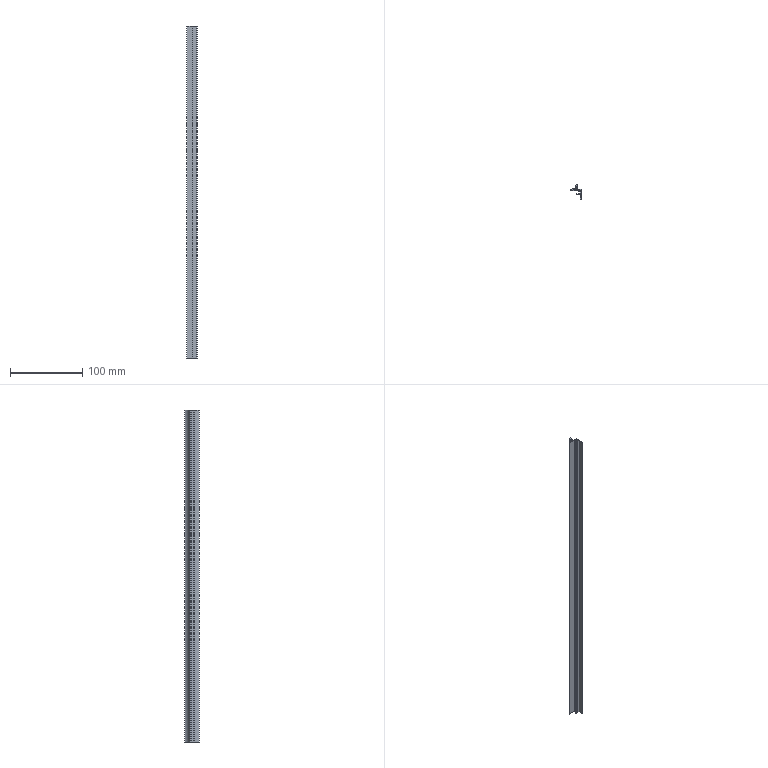Part | SolidWorks | features BaseBody 1, ICE 1, MoveFace 1 | 1 solid | 27 faces | box 14 x 20.3 x 461 mm | volume 23472 mm3 | plane 20 | cylinder 7 | commonest cylinder face diameters 0.387 x2 0.8 x2 0.4 x1 20 x1 22 x1
STEP:
#1=CARTESIAN_POINT('',(-5.304,-0.625,200.));
#2=VERTEX_POINT('',#1);
#3=CARTESIAN_POINT('',(-5.449,-0.8125,200.));
#4=VERTEX_POINT('',#3);
#5=CARTESIAN_POINT('',(-5.255,-0.8125,200.));
#6=DIRECTION('',(0.,0.,1.));
#7=DIRECTION('',(-1.,0.,0.));
#8=AXIS2_PLACEMENT_3D('',#5,#6,#7);
#9=CIRCLE('',#8,0.1937);
#10=EDGE_CURVE('',#2,#4,#9,.T.);
#11=ORIENTED_EDGE('',*,*,#10,.T.);
#12=CARTESIAN_POINT('',(-5.449,-0.8125,-261.));
#13=VERTEX_POINT('',#12);
#14=CARTESIAN_POINT('',(-5.449,-0.8125,230.));
#15=DIRECTION('',(0.,0.,-1.));
#16=VECTOR('',#15,1000.);
#17=LINE('',#14,#16);
#18=EDGE_CURVE('',#4,#13,#17,.T.);
#19=ORIENTED_EDGE('',*,*,#18,.T.);
#20=CARTESIAN_POINT('',(-5.304,-0.625,-261.));
#21=VERTEX_POINT('',#20);
#22=CARTESIAN_POINT('',(-5.255,-0.8125,-261.));
#23=DIRECTION('',(0.,0.,-1.));
#24=DIRECTION('',(1.,0.,0.));
#25=AXIS2_PLACEMENT_3D('',#22,#23,#24);
#26=CIRCLE('',#25,0.1937);
#27=EDGE_CURVE('',#13,#21,#26,.T.);
#28=ORIENTED_EDGE('',*,*,#27,.T.);
#29=CARTESIAN_POINT('',(-5.304,-0.625,230.));
#30=DIRECTION('',(0.,0.,-1.));
#31=VECTOR('',#30,1000.);
#32=LINE('',#29,#31);
#33=EDGE_CURVE('',#2,#21,#32,.T.);
#34=ORIENTED_EDGE('',*,*,#33,.F.);
#35=EDGE_LOOP('',(#11,#19,#28,#34));
#36=FACE_OUTER_BOUND('',#35,.T.);
#37=CARTESIAN_POINT('',(-5.255,-0.8125,230.));
#38=DIRECTION('',(0.,0.,-1.));
#39=DIRECTION('',(-1.,0.,0.));
#40=AXIS2_PLACEMENT_3D('',#37,#38,#39);
#41=CYLINDRICAL_SURFACE('',#40,0.1937);
#42=ADVANCED_FACE('',(#36),#41,.F.);
#43=CARTESIAN_POINT('',(5.,-1.,-261.));
#44=VERTEX_POINT('',#43);
#45=CARTESIAN_POINT('',(5.,-14.3,-261.));
#46=VERTEX_POINT('',#45);
#47=CARTESIAN_POINT('',(5.,29.623,-261.));
#48=DIRECTION('',(0.,-1.,0.));
#49=VECTOR('',#48,1000.);
#50=LINE('',#47,#49);
#51=EDGE_CURVE('',#44,#46,#50,.T.);
#52=ORIENTED_EDGE('',*,*,#51,.F.);
#53=CARTESIAN_POINT('',(5.,-1.,200.));
#54=VERTEX_POINT('',#53);
#55=CARTESIAN_POINT('',(5.,-1.,230.));
#56=DIRECTION('',(0.,0.,-1.));
#57=VECTOR('',#56,1000.);
#58=LINE('',#55,#57);
#59=EDGE_CURVE('',#54,#44,#58,.T.);
#60=ORIENTED_EDGE('',*,*,#59,.F.);
#61=CARTESIAN_POINT('',(5.,-14.3,200.));
#62=VERTEX_POINT('',#61);
#63=CARTESIAN_POINT('',(5.,-14.3,200.));
#64=DIRECTION('',(0.,1.,0.));
#65=VECTOR('',#64,1000.);
#66=LINE('',#63,#65);
#67=EDGE_CURVE('',#62,#54,#66,.T.);
#68=ORIENTED_EDGE('',*,*,#67,.F.);
#69=CARTESIAN_POINT('',(5.,-14.3,230.));
#70=DIRECTION('',(0.,0.,1.));
#71=VECTOR('',#70,1000.);
#72=LINE('',#69,#71);
#73=EDGE_CURVE('',#46,#62,#72,.T.);
#74=ORIENTED_EDGE('',*,*,#73,.F.);
#75=EDGE_LOOP('',(#52,#60,#68,#74));
#76=FACE_OUTER_BOUND('',#75,.T.);
#77=CARTESIAN_POINT('',(5.,-14.3,230.));
#78=DIRECTION('',(-1.,0.,0.));
#79=DIRECTION('',(0.,0.,1.));
#80=AXIS2_PLACEMENT_3D('',#77,#78,#79);
#81=PLANE('',#80);
#82=ADVANCED_FACE('',(#76),#81,.F.);
#83=CARTESIAN_POINT('',(-9.,-2.,-261.));
#84=VERTEX_POINT('',#83);
#85=CARTESIAN_POINT('',(-9.,-2.,200.));
#86=VERTEX_POINT('',#85);
#87=CARTESIAN_POINT('',(-9.,-2.,230.));
#88=DIRECTION('',(0.,0.,1.));
#89=VECTOR('',#88,1000.);
#90=LINE('',#87,#89);
#91=EDGE_CURVE('',#84,#86,#90,.T.);
#92=ORIENTED_EDGE('',*,*,#91,.F.);
#93=CARTESIAN_POINT('',(0.9,-2.,-261.));
#94=VERTEX_POINT('',#93);
#95=CARTESIAN_POINT('',(5.,-2.,-261.));
#96=DIRECTION('',(-1.,0.,0.));
#97=VECTOR('',#96,1000.);
#98=LINE('',#95,#97);
#99=EDGE_CURVE('',#94,#84,#98,.T.);
#100=ORIENTED_EDGE('',*,*,#99,.F.);
#101=CARTESIAN_POINT('',(0.9,-2.,200.));
#102=VERTEX_POINT('',#101);
#103=CARTESIAN_POINT('',(0.9,-2.,230.));
#104=DIRECTION('',(0.,0.,-1.));
#105=VECTOR('',#104,1000.);
#106=LINE('',#103,#105);
#107=EDGE_CURVE('',#102,#94,#106,.T.);
#108=ORIENTED_EDGE('',*,*,#107,.F.);
#109=CARTESIAN_POINT('',(5.,-2.,200.));
#110=DIRECTION('',(1.,0.,0.));
#111=VECTOR('',#110,1000.);
#112=LINE('',#109,#111);
#113=EDGE_CURVE('',#86,#102,#112,.T.);
#114=ORIENTED_EDGE('',*,*,#113,.F.);
#115=EDGE_LOOP('',(#92,#100,#108,#114));
#116=FACE_OUTER_BOUND('',#115,.T.);
#117=CARTESIAN_POINT('',(-9.,-2.,230.));
#118=DIRECTION('',(0.,1.,0.));
#119=DIRECTION('',(0.,0.,1.));
#120=AXIS2_PLACEMENT_3D('',#117,#118,#119);
#121=PLANE('',#120);
#122=ADVANCED_FACE('',(#116),#121,.F.);
#123=CARTESIAN_POINT('',(4.,-6.,200.));
#124=VERTEX_POINT('',#123);
#125=CARTESIAN_POINT('',(4.,-3.,200.));
#126=VERTEX_POINT('',#125);
#127=CARTESIAN_POINT('',(4.,29.623,200.));
#128=DIRECTION('',(0.,1.,0.));
#129=VECTOR('',#128,1000.);
#130=LINE('',#127,#129);
#131=EDGE_CURVE('',#124,#126,#130,.T.);
#132=ORIENTED_EDGE('',*,*,#131,.F.);
#133=CARTESIAN_POINT('',(1.,-6.,200.));
#134=VERTEX_POINT('',#133);
#135=CARTESIAN_POINT('',(5.,-6.,200.));
#136=DIRECTION('',(1.,0.,0.));
#137=VECTOR('',#136,1000.);
#138=LINE('',#135,#137);
#139=EDGE_CURVE('',#134,#124,#138,.T.);
#140=ORIENTED_EDGE('',*,*,#139,.F.);
#141=CARTESIAN_POINT('',(1.,-6.7,200.));
#142=VERTEX_POINT('',#141);
#143=CARTESIAN_POINT('',(1.,-6.,200.));
#144=DIRECTION('',(0.,-1.,0.));
#145=VECTOR('',#144,1000.);
#146=LINE('',#143,#145);
#147=EDGE_CURVE('',#134,#142,#146,.T.);
#148=ORIENTED_EDGE('',*,*,#147,.T.);
#149=CARTESIAN_POINT('',(-1.7,-6.7,200.));
#150=VERTEX_POINT('',#149);
#151=CARTESIAN_POINT('',(5.,-6.7,200.));
#152=DIRECTION('',(1.,0.,0.));
#153=VECTOR('',#152,1000.);
#154=LINE('',#151,#153);
#155=EDGE_CURVE('',#150,#142,#154,.T.);
#156=ORIENTED_EDGE('',*,*,#155,.F.);
#157=CARTESIAN_POINT('',(-1.7,-7.7,200.));
#158=VERTEX_POINT('',#157);
#159=CARTESIAN_POINT('',(-1.7,-6.7,200.));
#160=DIRECTION('',(0.,-1.,0.));
#161=VECTOR('',#160,1000.);
#162=LINE('',#159,#161);
#163=EDGE_CURVE('',#150,#158,#162,.T.);
#164=ORIENTED_EDGE('',*,*,#163,.T.);
#165=CARTESIAN_POINT('',(4.,-7.7,200.));
#166=VERTEX_POINT('',#165);
#167=CARTESIAN_POINT('',(5.,-7.7,200.));
#168=DIRECTION('',(-1.,0.,0.));
#169=VECTOR('',#168,1000.);
#170=LINE('',#167,#169);
#171=EDGE_CURVE('',#166,#158,#170,.T.);
#172=ORIENTED_EDGE('',*,*,#171,.F.);
#173=CARTESIAN_POINT('',(4.,-14.3,200.));
#174=VERTEX_POINT('',#173);
#175=CARTESIAN_POINT('',(4.,29.623,200.));
#176=DIRECTION('',(0.,1.,0.));
#177=VECTOR('',#176,1000.);
#178=LINE('',#175,#177);
#179=EDGE_CURVE('',#174,#166,#178,.T.);
#180=ORIENTED_EDGE('',*,*,#179,.F.);
#181=CARTESIAN_POINT('',(5.,-14.3,200.));
#182=DIRECTION('',(-1.,0.,0.));
#183=VECTOR('',#182,1000.);
#184=LINE('',#181,#183);
#185=EDGE_CURVE('',#62,#174,#184,.T.);
#186=ORIENTED_EDGE('',*,*,#185,.F.);
#187=ORIENTED_EDGE('',*,*,#67,.T.);
#188=CARTESIAN_POINT('',(-5.207,-1.,200.));
#189=VERTEX_POINT('',#188);
#190=CARTESIAN_POINT('',(5.,-1.,200.));
#191=DIRECTION('',(1.,0.,0.));
#192=VECTOR('',#191,1000.);
#193=LINE('',#190,#192);
#194=EDGE_CURVE('',#189,#54,#193,.T.);
#195=ORIENTED_EDGE('',*,*,#194,.F.);
#196=CARTESIAN_POINT('',(-5.255,-0.8125,200.));
#197=DIRECTION('',(0.,0.,1.));
#198=DIRECTION('',(-1.,0.,0.));
#199=AXIS2_PLACEMENT_3D('',#196,#197,#198);
#200=CIRCLE('',#199,0.1937);
#201=EDGE_CURVE('',#4,#189,#200,.T.);
#202=ORIENTED_EDGE('',*,*,#201,.F.);
#203=ORIENTED_EDGE('',*,*,#10,.F.);
#204=CARTESIAN_POINT('',(-1.368,3.063,200.));
#205=VERTEX_POINT('',#204);
#206=CARTESIAN_POINT('',(-10.628,9.,200.));
#207=DIRECTION('',(0.,0.,1.));
#208=DIRECTION('',(-1.,0.,0.));
#209=AXIS2_PLACEMENT_3D('',#206,#207,#208);
#210=CIRCLE('',#209,11.);
#211=EDGE_CURVE('',#2,#205,#210,.T.);
#212=ORIENTED_EDGE('',*,*,#211,.T.);
#213=CARTESIAN_POINT('',(-1.,2.955,200.));
#214=VERTEX_POINT('',#213);
#215=CARTESIAN_POINT('',(-1.2,2.955,200.));
#216=DIRECTION('',(0.,0.,1.));
#217=DIRECTION('',(-1.,0.,0.));
#218=AXIS2_PLACEMENT_3D('',#215,#216,#217);
#219=CIRCLE('',#218,0.2);
#220=EDGE_CURVE('',#214,#205,#219,.T.);
#221=ORIENTED_EDGE('',*,*,#220,.F.);
#222=CARTESIAN_POINT('',(-1.,1.5,200.));
#223=VERTEX_POINT('',#222);
#224=CARTESIAN_POINT('',(-1.,2.955,200.));
#225=DIRECTION('',(0.,1.,0.));
#226=VECTOR('',#225,1000.);
#227=LINE('',#224,#226);
#228=EDGE_CURVE('',#223,#214,#227,.T.);
#229=ORIENTED_EDGE('',*,*,#228,.F.);
#230=CARTESIAN_POINT('',(0.,1.5,200.));
#231=VERTEX_POINT('',#230);
#232=CARTESIAN_POINT('',(-1.,1.5,200.));
#233=DIRECTION('',(-1.,0.,0.));
#234=VECTOR('',#233,1000.);
#235=LINE('',#232,#234);
#236=EDGE_CURVE('',#231,#223,#235,.T.);
#237=ORIENTED_EDGE('',*,*,#236,.F.);
#238=CARTESIAN_POINT('',(0.,6.,200.));
#239=VERTEX_POINT('',#238);
#240=CARTESIAN_POINT('',(0.,1.5,200.));
#241=DIRECTION('',(0.,-1.,0.));
#242=VECTOR('',#241,1000.);
#243=LINE('',#240,#242);
#244=EDGE_CURVE('',#239,#231,#243,.T.);
#245=ORIENTED_EDGE('',*,*,#244,.F.);
#246=CARTESIAN_POINT('',(-0.8,6.,200.));
#247=VERTEX_POINT('',#246);
#248=CARTESIAN_POINT('',(0.,6.,200.));
#249=DIRECTION('',(1.,0.,0.));
#250=VECTOR('',#249,1000.);
#251=LINE('',#248,#250);
#252=EDGE_CURVE('',#247,#239,#251,.T.);
#253=ORIENTED_EDGE('',*,*,#252,.F.);
#254=CARTESIAN_POINT('',(-1.178,5.731,200.));
#255=VERTEX_POINT('',#254);
#256=CARTESIAN_POINT('',(-0.8,5.6,200.));
#257=DIRECTION('',(0.,0.,1.));
#258=DIRECTION('',(-1.,0.,0.));
#259=AXIS2_PLACEMENT_3D('',#256,#257,#258);
#260=CIRCLE('',#259,0.4);
#261=EDGE_CURVE('',#247,#255,#260,.T.);
#262=ORIENTED_EDGE('',*,*,#261,.T.);
#263=CARTESIAN_POINT('',(-8.678,-0.8077,200.));
#264=VERTEX_POINT('',#263);
#265=CARTESIAN_POINT('',(-10.628,9.,200.));
#266=DIRECTION('',(0.,0.,1.));
#267=DIRECTION('',(-1.,0.,0.));
#268=AXIS2_PLACEMENT_3D('',#265,#266,#267);
#269=CIRCLE('',#268,10.);
#270=EDGE_CURVE('',#264,#255,#269,.T.);
#271=ORIENTED_EDGE('',*,*,#270,.F.);
#272=CARTESIAN_POINT('',(-9.,-1.2,200.));
#273=VERTEX_POINT('',#272);
#274=CARTESIAN_POINT('',(-8.6,-1.2,200.));
#275=DIRECTION('',(0.,0.,1.));
#276=DIRECTION('',(-1.,0.,0.));
#277=AXIS2_PLACEMENT_3D('',#274,#275,#276);
#278=CIRCLE('',#277,0.4);
#279=EDGE_CURVE('',#264,#273,#278,.T.);
#280=ORIENTED_EDGE('',*,*,#279,.T.);
#281=CARTESIAN_POINT('',(-9.,8.,200.));
#282=DIRECTION('',(0.,-1.,0.));
#283=VECTOR('',#282,1000.);
#284=LINE('',#281,#283);
#285=EDGE_CURVE('',#273,#86,#284,.T.);
#286=ORIENTED_EDGE('',*,*,#285,.T.);
#287=ORIENTED_EDGE('',*,*,#113,.T.);
#288=CARTESIAN_POINT('',(0.9,-3.,200.));
#289=VERTEX_POINT('',#288);
#290=CARTESIAN_POINT('',(0.9,29.623,200.));
#291=DIRECTION('',(0.,1.,0.));
#292=VECTOR('',#291,1000.);
#293=LINE('',#290,#292);
#294=EDGE_CURVE('',#289,#102,#293,.T.);
#295=ORIENTED_EDGE('',*,*,#294,.F.);
#296=CARTESIAN_POINT('',(5.,-3.,200.));
#297=DIRECTION('',(-1.,0.,0.));
#298=VECTOR('',#297,1000.);
#299=LINE('',#296,#298);
#300=EDGE_CURVE('',#126,#289,#299,.T.);
#301=ORIENTED_EDGE('',*,*,#300,.F.);
#302=EDGE_LOOP('',(#132,#140,#148,#156,#164,#172,#180,#186,#187,#195,#202,#203,#212,#221,#229,#237,#245,#253,#262,#271,#280,#286,#287,#295,#301));
#303=FACE_OUTER_BOUND('',#302,.T.);
#304=CARTESIAN_POINT('',(5.,29.623,200.));
#305=DIRECTION('',(0.,0.,-1.));
#306=DIRECTION('',(-1.,0.,0.));
#307=AXIS2_PLACEMENT_3D('',#304,#305,#306);
#308=PLANE('',#307);
#309=ADVANCED_FACE('',(#303),#308,.F.);
#310=ORIENTED_EDGE('',*,*,#185,.T.);
#311=CARTESIAN_POINT('',(4.,-14.3,-261.));
#312=VERTEX_POINT('',#311);
#313=CARTESIAN_POINT('',(4.,-14.3,230.));
#314=DIRECTION('',(0.,0.,1.));
#315=VECTOR('',#314,1000.);
#316=LINE('',#313,#315);
#317=EDGE_CURVE('',#312,#174,#316,.T.);
#318=ORIENTED_EDGE('',*,*,#317,.F.);
#319=CARTESIAN_POINT('',(5.,-14.3,-261.));
#320=DIRECTION('',(-1.,0.,0.));
#321=VECTOR('',#320,1000.);
#322=LINE('',#319,#321);
#323=EDGE_CURVE('',#46,#312,#322,.T.);
#324=ORIENTED_EDGE('',*,*,#323,.F.);
#325=ORIENTED_EDGE('',*,*,#73,.T.);
#326=EDGE_LOOP('',(#310,#318,#324,#325));
#327=FACE_OUTER_BOUND('',#326,.T.);
#328=CARTESIAN_POINT('',(4.,-14.3,230.));
#329=DIRECTION('',(0.,1.,0.));
#330=DIRECTION('',(0.,0.,1.));
#331=AXIS2_PLACEMENT_3D('',#328,#329,#330);
#332=PLANE('',#331);
#333=ADVANCED_FACE('',(#327),#332,.F.);
#334=ORIENTED_EDGE('',*,*,#51,.T.);
#335=ORIENTED_EDGE('',*,*,#323,.T.);
#336=CARTESIAN_POINT('',(4.,-7.7,-261.));
#337=VERTEX_POINT('',#336);
#338=CARTESIAN_POINT('',(4.,-7.7,-261.));
#339=DIRECTION('',(0.,-1.,0.));
#340=VECTOR('',#339,1000.);
#341=LINE('',#338,#340);
#342=EDGE_CURVE('',#337,#312,#341,.T.);
#343=ORIENTED_EDGE('',*,*,#342,.F.);
#344=CARTESIAN_POINT('',(-1.7,-7.7,-261.));
#345=VERTEX_POINT('',#344);
#346=CARTESIAN_POINT('',(-1.7,-7.7,-261.));
#347=DIRECTION('',(1.,0.,0.));
#348=VECTOR('',#347,1000.);
#349=LINE('',#346,#348);
#350=EDGE_CURVE('',#345,#337,#349,.T.);
#351=ORIENTED_EDGE('',*,*,#350,.F.);
#352=CARTESIAN_POINT('',(-1.7,-6.7,-261.));
#353=VERTEX_POINT('',#352);
#354=CARTESIAN_POINT('',(-1.7,29.623,-261.));
#355=DIRECTION('',(0.,1.,0.));
#356=VECTOR('',#355,1000.);
#357=LINE('',#354,#356);
#358=EDGE_CURVE('',#345,#353,#357,.T.);
#359=ORIENTED_EDGE('',*,*,#358,.T.);
#360=CARTESIAN_POINT('',(1.,-6.7,-261.));
#361=VERTEX_POINT('',#360);
#362=CARTESIAN_POINT('',(1.,-6.7,-261.));
#363=DIRECTION('',(-1.,0.,0.));
#364=VECTOR('',#363,1000.);
#365=LINE('',#362,#364);
#366=EDGE_CURVE('',#361,#353,#365,.T.);
#367=ORIENTED_EDGE('',*,*,#366,.F.);
#368=CARTESIAN_POINT('',(1.,-6.,-261.));
#369=VERTEX_POINT('',#368);
#370=CARTESIAN_POINT('',(1.,29.623,-261.));
#371=DIRECTION('',(0.,1.,0.));
#372=VECTOR('',#371,1000.);
#373=LINE('',#370,#372);
#374=EDGE_CURVE('',#361,#369,#373,.T.);
#375=ORIENTED_EDGE('',*,*,#374,.T.);
#376=CARTESIAN_POINT('',(4.,-6.,-261.));
#377=VERTEX_POINT('',#376);
#378=CARTESIAN_POINT('',(4.,-6.,-261.));
#379=DIRECTION('',(-1.,0.,0.));
#380=VECTOR('',#379,1000.);
#381=LINE('',#378,#380);
#382=EDGE_CURVE('',#377,#369,#381,.T.);
#383=ORIENTED_EDGE('',*,*,#382,.F.);
#384=CARTESIAN_POINT('',(4.,-3.,-261.));
#385=VERTEX_POINT('',#384);
#386=CARTESIAN_POINT('',(4.,-3.,-261.));
#387=DIRECTION('',(0.,-1.,0.));
#388=VECTOR('',#387,1000.);
#389=LINE('',#386,#388);
#390=EDGE_CURVE('',#385,#377,#389,.T.);
#391=ORIENTED_EDGE('',*,*,#390,.F.);
#392=CARTESIAN_POINT('',(0.9,-3.,-261.));
#393=VERTEX_POINT('',#392);
#394=CARTESIAN_POINT('',(0.9,-3.,-261.));
#395=DIRECTION('',(1.,0.,0.));
#396=VECTOR('',#395,1000.);
#397=LINE('',#394,#396);
#398=EDGE_CURVE('',#393,#385,#397,.T.);
#399=ORIENTED_EDGE('',*,*,#398,.F.);
#400=CARTESIAN_POINT('',(0.9,-2.,-261.));
#401=DIRECTION('',(0.,-1.,0.));
#402=VECTOR('',#401,1000.);
#403=LINE('',#400,#402);
#404=EDGE_CURVE('',#94,#393,#403,.T.);
#405=ORIENTED_EDGE('',*,*,#404,.F.);
#406=ORIENTED_EDGE('',*,*,#99,.T.);
#407=CARTESIAN_POINT('',(-9.,-1.2,-261.));
#408=VERTEX_POINT('',#407);
#409=CARTESIAN_POINT('',(-9.,-1.2,-261.));
#410=DIRECTION('',(0.,-1.,0.));
#411=VECTOR('',#410,1000.);
#412=LINE('',#409,#411);
#413=EDGE_CURVE('',#408,#84,#412,.T.);
#414=ORIENTED_EDGE('',*,*,#413,.F.);
#415=CARTESIAN_POINT('',(-8.678,-0.8077,-261.));
#416=VERTEX_POINT('',#415);
#417=CARTESIAN_POINT('',(-8.6,-1.2,-261.));
#418=DIRECTION('',(0.,0.,-1.));
#419=DIRECTION('',(1.,0.,0.));
#420=AXIS2_PLACEMENT_3D('',#417,#418,#419);
#421=CIRCLE('',#420,0.4);
#422=EDGE_CURVE('',#408,#416,#421,.T.);
#423=ORIENTED_EDGE('',*,*,#422,.T.);
#424=CARTESIAN_POINT('',(-1.178,5.731,-261.));
#425=VERTEX_POINT('',#424);
#426=CARTESIAN_POINT('',(-10.628,9.,-261.));
#427=DIRECTION('',(0.,0.,-1.));
#428=DIRECTION('',(1.,0.,0.));
#429=AXIS2_PLACEMENT_3D('',#426,#427,#428);
#430=CIRCLE('',#429,10.);
#431=EDGE_CURVE('',#425,#416,#430,.T.);
#432=ORIENTED_EDGE('',*,*,#431,.F.);
#433=CARTESIAN_POINT('',(-0.8,6.,-261.));
#434=VERTEX_POINT('',#433);
#435=CARTESIAN_POINT('',(-0.8,5.6,-261.));
#436=DIRECTION('',(0.,0.,-1.));
#437=DIRECTION('',(1.,0.,0.));
#438=AXIS2_PLACEMENT_3D('',#435,#436,#437);
#439=CIRCLE('',#438,0.4);
#440=EDGE_CURVE('',#425,#434,#439,.T.);
#441=ORIENTED_EDGE('',*,*,#440,.T.);
#442=CARTESIAN_POINT('',(0.,6.,-261.));
#443=VERTEX_POINT('',#442);
#444=CARTESIAN_POINT('',(0.,6.,-261.));
#445=DIRECTION('',(-1.,0.,0.));
#446=VECTOR('',#445,1000.);
#447=LINE('',#444,#446);
#448=EDGE_CURVE('',#443,#434,#447,.T.);
#449=ORIENTED_EDGE('',*,*,#448,.F.);
#450=CARTESIAN_POINT('',(0.,1.5,-261.));
#451=VERTEX_POINT('',#450);
#452=CARTESIAN_POINT('',(0.,1.5,-261.));
#453=DIRECTION('',(0.,1.,0.));
#454=VECTOR('',#453,1000.);
#455=LINE('',#452,#454);
#456=EDGE_CURVE('',#451,#443,#455,.T.);
#457=ORIENTED_EDGE('',*,*,#456,.F.);
#458=CARTESIAN_POINT('',(-1.,1.5,-261.));
#459=VERTEX_POINT('',#458);
#460=CARTESIAN_POINT('',(-1.,1.5,-261.));
#461=DIRECTION('',(1.,0.,0.));
#462=VECTOR('',#461,1000.);
#463=LINE('',#460,#462);
#464=EDGE_CURVE('',#459,#451,#463,.T.);
#465=ORIENTED_EDGE('',*,*,#464,.F.);
#466=CARTESIAN_POINT('',(-1.,2.955,-261.));
#467=VERTEX_POINT('',#466);
#468=CARTESIAN_POINT('',(-1.,2.955,-261.));
#469=DIRECTION('',(0.,-1.,0.));
#470=VECTOR('',#469,1000.);
#471=LINE('',#468,#470);
#472=EDGE_CURVE('',#467,#459,#471,.T.);
#473=ORIENTED_EDGE('',*,*,#472,.F.);
#474=CARTESIAN_POINT('',(-1.368,3.063,-261.));
#475=VERTEX_POINT('',#474);
#476=CARTESIAN_POINT('',(-1.2,2.955,-261.));
#477=DIRECTION('',(0.,0.,-1.));
#478=DIRECTION('',(1.,0.,0.));
#479=AXIS2_PLACEMENT_3D('',#476,#477,#478);
#480=CIRCLE('',#479,0.2);
#481=EDGE_CURVE('',#475,#467,#480,.T.);
#482=ORIENTED_EDGE('',*,*,#481,.F.);
#483=CARTESIAN_POINT('',(-10.628,9.,-261.));
#484=DIRECTION('',(0.,0.,-1.));
#485=DIRECTION('',(1.,0.,0.));
#486=AXIS2_PLACEMENT_3D('',#483,#484,#485);
#487=CIRCLE('',#486,11.);
#488=EDGE_CURVE('',#475,#21,#487,.T.);
#489=ORIENTED_EDGE('',*,*,#488,.T.);
#490=ORIENTED_EDGE('',*,*,#27,.F.);
#491=CARTESIAN_POINT('',(-5.207,-1.,-261.));
#492=VERTEX_POINT('',#491);
#493=CARTESIAN_POINT('',(-5.255,-0.8125,-261.));
#494=DIRECTION('',(0.,0.,-1.));
#495=DIRECTION('',(1.,0.,0.));
#496=AXIS2_PLACEMENT_3D('',#493,#494,#495);
#497=CIRCLE('',#496,0.1937);
#498=EDGE_CURVE('',#492,#13,#497,.T.);
#499=ORIENTED_EDGE('',*,*,#498,.F.);
#500=CARTESIAN_POINT('',(5.,-1.,-261.));
#501=DIRECTION('',(-1.,0.,0.));
#502=VECTOR('',#501,1000.);
#503=LINE('',#500,#502);
#504=EDGE_CURVE('',#44,#492,#503,.T.);
#505=ORIENTED_EDGE('',*,*,#504,.F.);
#506=EDGE_LOOP('',(#334,#335,#343,#351,#359,#367,#375,#383,#391,#399,#405,#406,#414,#423,#432,#441,#449,#457,#465,#473,#482,#489,#490,#499,#505));
#507=FACE_OUTER_BOUND('',#506,.T.);
#508=CARTESIAN_POINT('',(5.,29.623,-261.));
#509=DIRECTION('',(0.,0.,1.));
#510=DIRECTION('',(1.,0.,0.));
#511=AXIS2_PLACEMENT_3D('',#508,#509,#510);
#512=PLANE('',#511);
#513=ADVANCED_FACE('',(#507),#512,.F.);
#514=ORIENTED_EDGE('',*,*,#59,.T.);
#515=ORIENTED_EDGE('',*,*,#504,.T.);
#516=CARTESIAN_POINT('',(-5.207,-1.,230.));
#517=DIRECTION('',(0.,0.,-1.));
#518=VECTOR('',#517,1000.);
#519=LINE('',#516,#518);
#520=EDGE_CURVE('',#189,#492,#519,.T.);
#521=ORIENTED_EDGE('',*,*,#520,.F.);
#522=ORIENTED_EDGE('',*,*,#194,.T.);
#523=EDGE_LOOP('',(#514,#515,#521,#522));
#524=FACE_OUTER_BOUND('',#523,.T.);
#525=CARTESIAN_POINT('',(5.,-1.,230.));
#526=DIRECTION('',(0.,-1.,0.));
#527=DIRECTION('',(0.,0.,-1.));
#528=AXIS2_PLACEMENT_3D('',#525,#526,#527);
#529=PLANE('',#528);
#530=ADVANCED_FACE('',(#524),#529,.F.);
#531=CARTESIAN_POINT('',(-9.,-1.2,230.));
#532=DIRECTION('',(0.,0.,1.));
#533=VECTOR('',#532,1000.);
#534=LINE('',#531,#533);
#535=EDGE_CURVE('',#408,#273,#534,.T.);
#536=ORIENTED_EDGE('',*,*,#535,.F.);
#537=ORIENTED_EDGE('',*,*,#413,.T.);
#538=ORIENTED_EDGE('',*,*,#91,.T.);
#539=ORIENTED_EDGE('',*,*,#285,.F.);
#540=EDGE_LOOP('',(#536,#537,#538,#539));
#541=FACE_OUTER_BOUND('',#540,.T.);
#542=CARTESIAN_POINT('',(-9.,-1.2,230.));
#543=DIRECTION('',(1.,0.,0.));
#544=DIRECTION('',(0.,0.,-1.));
#545=AXIS2_PLACEMENT_3D('',#542,#543,#544);
#546=PLANE('',#545);
#547=ADVANCED_FACE('',(#541),#546,.F.);
#548=ORIENTED_EDGE('',*,*,#294,.T.);
#549=ORIENTED_EDGE('',*,*,#107,.T.);
#550=ORIENTED_EDGE('',*,*,#404,.T.);
#551=CARTESIAN_POINT('',(0.9,-3.,230.));
#552=DIRECTION('',(0.,0.,-1.));
#553=VECTOR('',#552,1000.);
#554=LINE('',#551,#553);
#555=EDGE_CURVE('',#289,#393,#554,.T.);
#556=ORIENTED_EDGE('',*,*,#555,.F.);
#557=EDGE_LOOP('',(#548,#549,#550,#556));
#558=FACE_OUTER_BOUND('',#557,.T.);
#559=CARTESIAN_POINT('',(0.9,-2.,230.));
#560=DIRECTION('',(1.,0.,0.));
#561=DIRECTION('',(0.,0.,-1.));
#562=AXIS2_PLACEMENT_3D('',#559,#560,#561);
#563=PLANE('',#562);
#564=ADVANCED_FACE('',(#558),#563,.F.);
#565=ORIENTED_EDGE('',*,*,#300,.T.);
#566=ORIENTED_EDGE('',*,*,#555,.T.);
#567=ORIENTED_EDGE('',*,*,#398,.T.);
#568=CARTESIAN_POINT('',(4.,-3.,230.));
#569=DIRECTION('',(0.,0.,-1.));
#570=VECTOR('',#569,1000.);
#571=LINE('',#568,#570);
#572=EDGE_CURVE('',#126,#385,#571,.T.);
#573=ORIENTED_EDGE('',*,*,#572,.F.);
#574=EDGE_LOOP('',(#565,#566,#567,#573));
#575=FACE_OUTER_BOUND('',#574,.T.);
#576=CARTESIAN_POINT('',(0.9,-3.,230.));
#577=DIRECTION('',(0.,1.,0.));
#578=DIRECTION('',(0.,0.,1.));
#579=AXIS2_PLACEMENT_3D('',#576,#577,#578);
#580=PLANE('',#579);
#581=ADVANCED_FACE('',(#575),#580,.F.);
#582=ORIENTED_EDGE('',*,*,#131,.T.);
#583=ORIENTED_EDGE('',*,*,#572,.T.);
#584=ORIENTED_EDGE('',*,*,#390,.T.);
#585=CARTESIAN_POINT('',(4.,-6.,230.));
#586=DIRECTION('',(0.,0.,-1.));
#587=VECTOR('',#586,1000.);
#588=LINE('',#585,#587);
#589=EDGE_CURVE('',#124,#377,#588,.T.);
#590=ORIENTED_EDGE('',*,*,#589,.F.);
#591=EDGE_LOOP('',(#582,#583,#584,#590));
#592=FACE_OUTER_BOUND('',#591,.T.);
#593=CARTESIAN_POINT('',(4.,-3.,230.));
#594=DIRECTION('',(1.,0.,0.));
#595=DIRECTION('',(0.,0.,-1.));
#596=AXIS2_PLACEMENT_3D('',#593,#594,#595);
#597=PLANE('',#596);
#598=ADVANCED_FACE('',(#592),#597,.F.);
#599=ORIENTED_EDGE('',*,*,#139,.T.);
#600=ORIENTED_EDGE('',*,*,#589,.T.);
#601=ORIENTED_EDGE('',*,*,#382,.T.);
#602=CARTESIAN_POINT('',(1.,-6.,230.));
#603=DIRECTION('',(0.,0.,-1.));
#604=VECTOR('',#603,1000.);
#605=LINE('',#602,#604);
#606=EDGE_CURVE('',#134,#369,#605,.T.);
#607=ORIENTED_EDGE('',*,*,#606,.F.);
#608=EDGE_LOOP('',(#599,#600,#601,#607));
#609=FACE_OUTER_BOUND('',#608,.T.);
#610=CARTESIAN_POINT('',(4.,-6.,230.));
#611=DIRECTION('',(0.,-1.,0.));
#612=DIRECTION('',(0.,0.,-1.));
#613=AXIS2_PLACEMENT_3D('',#610,#611,#612);
#614=PLANE('',#613);
#615=ADVANCED_FACE('',(#609),#614,.F.);
#616=ORIENTED_EDGE('',*,*,#155,.T.);
#617=CARTESIAN_POINT('',(1.,-6.7,230.));
#618=DIRECTION('',(0.,0.,1.));
#619=VECTOR('',#618,1000.);
#620=LINE('',#617,#619);
#621=EDGE_CURVE('',#361,#142,#620,.T.);
#622=ORIENTED_EDGE('',*,*,#621,.F.);
#623=ORIENTED_EDGE('',*,*,#366,.T.);
#624=CARTESIAN_POINT('',(-1.7,-6.7,230.));
#625=DIRECTION('',(0.,0.,-1.));
#626=VECTOR('',#625,1000.);
#627=LINE('',#624,#626);
#628=EDGE_CURVE('',#150,#353,#627,.T.);
#629=ORIENTED_EDGE('',*,*,#628,.F.);
#630=EDGE_LOOP('',(#616,#622,#623,#629));
#631=FACE_OUTER_BOUND('',#630,.T.);
#632=CARTESIAN_POINT('',(1.,-6.7,230.));
#633=DIRECTION('',(0.,-1.,0.));
#634=DIRECTION('',(0.,0.,-1.));
#635=AXIS2_PLACEMENT_3D('',#632,#633,#634);
#636=PLANE('',#635);
#637=ADVANCED_FACE('',(#631),#636,.F.);
#638=ORIENTED_EDGE('',*,*,#171,.T.);
#639=CARTESIAN_POINT('',(-1.7,-7.7,230.));
#640=DIRECTION('',(0.,0.,1.));
#641=VECTOR('',#640,1000.);
#642=LINE('',#639,#641);
#643=EDGE_CURVE('',#345,#158,#642,.T.);
#644=ORIENTED_EDGE('',*,*,#643,.F.);
#645=ORIENTED_EDGE('',*,*,#350,.T.);
#646=CARTESIAN_POINT('',(4.,-7.7,230.));
#647=DIRECTION('',(0.,0.,-1.));
#648=VECTOR('',#647,1000.);
#649=LINE('',#646,#648);
#650=EDGE_CURVE('',#166,#337,#649,.T.);
#651=ORIENTED_EDGE('',*,*,#650,.F.);
#652=EDGE_LOOP('',(#638,#644,#645,#651));
#653=FACE_OUTER_BOUND('',#652,.T.);
#654=CARTESIAN_POINT('',(-1.7,-7.7,230.));
#655=DIRECTION('',(0.,1.,0.));
#656=DIRECTION('',(0.,0.,1.));
#657=AXIS2_PLACEMENT_3D('',#654,#655,#656);
#658=PLANE('',#657);
#659=ADVANCED_FACE('',(#653),#658,.F.);
#660=ORIENTED_EDGE('',*,*,#179,.T.);
#661=ORIENTED_EDGE('',*,*,#650,.T.);
#662=ORIENTED_EDGE('',*,*,#342,.T.);
#663=ORIENTED_EDGE('',*,*,#317,.T.);
#664=EDGE_LOOP('',(#660,#661,#662,#663));
#665=FACE_OUTER_BOUND('',#664,.T.);
#666=CARTESIAN_POINT('',(4.,-7.7,230.));
#667=DIRECTION('',(1.,0.,0.));
#668=DIRECTION('',(0.,0.,-1.));
#669=AXIS2_PLACEMENT_3D('',#666,#667,#668);
#670=PLANE('',#669);
#671=ADVANCED_FACE('',(#665),#670,.F.);
#672=ORIENTED_EDGE('',*,*,#18,.F.);
#673=ORIENTED_EDGE('',*,*,#201,.T.);
#674=ORIENTED_EDGE('',*,*,#520,.T.);
#675=ORIENTED_EDGE('',*,*,#498,.T.);
#676=EDGE_LOOP('',(#672,#673,#674,#675));
#677=FACE_OUTER_BOUND('',#676,.T.);
#678=CARTESIAN_POINT('',(-5.255,-0.8125,230.));
#679=DIRECTION('',(0.,0.,-1.));
#680=DIRECTION('',(-1.,0.,0.));
#681=AXIS2_PLACEMENT_3D('',#678,#679,#680);
#682=CYLINDRICAL_SURFACE('',#681,0.1937);
#683=ADVANCED_FACE('',(#677),#682,.F.);
#684=CARTESIAN_POINT('',(-1.,2.955,230.));
#685=DIRECTION('',(0.,0.,1.));
#686=VECTOR('',#685,1000.);
#687=LINE('',#684,#686);
#688=EDGE_CURVE('',#467,#214,#687,.T.);
#689=ORIENTED_EDGE('',*,*,#688,.F.);
#690=ORIENTED_EDGE('',*,*,#472,.T.);
#691=CARTESIAN_POINT('',(-1.,1.5,230.));
#692=DIRECTION('',(0.,0.,-1.));
#693=VECTOR('',#692,1000.);
#694=LINE('',#691,#693);
#695=EDGE_CURVE('',#223,#459,#694,.T.);
#696=ORIENTED_EDGE('',*,*,#695,.F.);
#697=ORIENTED_EDGE('',*,*,#228,.T.);
#698=EDGE_LOOP('',(#689,#690,#696,#697));
#699=FACE_OUTER_BOUND('',#698,.T.);
#700=CARTESIAN_POINT('',(-1.,2.955,230.));
#701=DIRECTION('',(1.,0.,0.));
#702=DIRECTION('',(0.,0.,-1.));
#703=AXIS2_PLACEMENT_3D('',#700,#701,#702);
#704=PLANE('',#703);
#705=ADVANCED_FACE('',(#699),#704,.F.);
#706=ORIENTED_EDGE('',*,*,#488,.F.);
#707=CARTESIAN_POINT('',(-1.368,3.063,230.));
#708=DIRECTION('',(0.,0.,1.));
#709=VECTOR('',#708,1000.);
#710=LINE('',#707,#709);
#711=EDGE_CURVE('',#475,#205,#710,.T.);
#712=ORIENTED_EDGE('',*,*,#711,.T.);
#713=ORIENTED_EDGE('',*,*,#211,.F.);
#714=ORIENTED_EDGE('',*,*,#33,.T.);
#715=EDGE_LOOP('',(#706,#712,#713,#714));
#716=FACE_OUTER_BOUND('',#715,.T.);
#717=CARTESIAN_POINT('',(-10.628,9.,230.));
#718=DIRECTION('',(0.,0.,-1.));
#719=DIRECTION('',(-1.,0.,0.));
#720=AXIS2_PLACEMENT_3D('',#717,#718,#719);
#721=CYLINDRICAL_SURFACE('',#720,11.);
#722=ADVANCED_FACE('',(#716),#721,.T.);
#723=CARTESIAN_POINT('',(-1.178,5.731,230.));
#724=DIRECTION('',(0.,0.,1.));
#725=VECTOR('',#724,1000.);
#726=LINE('',#723,#725);
#727=EDGE_CURVE('',#425,#255,#726,.T.);
#728=ORIENTED_EDGE('',*,*,#727,.F.);
#729=ORIENTED_EDGE('',*,*,#431,.T.);
#730=CARTESIAN_POINT('',(-8.678,-0.8077,230.));
#731=DIRECTION('',(0.,0.,-1.));
#732=VECTOR('',#731,1000.);
#733=LINE('',#730,#732);
#734=EDGE_CURVE('',#264,#416,#733,.T.);
#735=ORIENTED_EDGE('',*,*,#734,.F.);
#736=ORIENTED_EDGE('',*,*,#270,.T.);
#737=EDGE_LOOP('',(#728,#729,#735,#736));
#738=FACE_OUTER_BOUND('',#737,.T.);
#739=CARTESIAN_POINT('',(-10.628,9.,230.));
#740=DIRECTION('',(0.,0.,-1.));
#741=DIRECTION('',(-1.,0.,0.));
#742=AXIS2_PLACEMENT_3D('',#739,#740,#741);
#743=CYLINDRICAL_SURFACE('',#742,10.);
#744=ADVANCED_FACE('',(#738),#743,.F.);
#745=CARTESIAN_POINT('',(0.,1.5,230.));
#746=DIRECTION('',(0.,0.,1.));
#747=VECTOR('',#746,1000.);
#748=LINE('',#745,#747);
#749=EDGE_CURVE('',#451,#231,#748,.T.);
#750=ORIENTED_EDGE('',*,*,#749,.F.);
#751=ORIENTED_EDGE('',*,*,#456,.T.);
#752=CARTESIAN_POINT('',(0.,6.,230.));
#753=DIRECTION('',(0.,0.,-1.));
#754=VECTOR('',#753,1000.);
#755=LINE('',#752,#754);
#756=EDGE_CURVE('',#239,#443,#755,.T.);
#757=ORIENTED_EDGE('',*,*,#756,.F.);
#758=ORIENTED_EDGE('',*,*,#244,.T.);
#759=EDGE_LOOP('',(#750,#751,#757,#758));
#760=FACE_OUTER_BOUND('',#759,.T.);
#761=CARTESIAN_POINT('',(0.,1.5,230.));
#762=DIRECTION('',(-1.,0.,0.));
#763=DIRECTION('',(0.,0.,1.));
#764=AXIS2_PLACEMENT_3D('',#761,#762,#763);
#765=PLANE('',#764);
#766=ADVANCED_FACE('',(#760),#765,.F.);
#767=ORIENTED_EDGE('',*,*,#422,.F.);
#768=ORIENTED_EDGE('',*,*,#535,.T.);
#769=ORIENTED_EDGE('',*,*,#279,.F.);
#770=ORIENTED_EDGE('',*,*,#734,.T.);
#771=EDGE_LOOP('',(#767,#768,#769,#770));
#772=FACE_OUTER_BOUND('',#771,.T.);
#773=CARTESIAN_POINT('',(-8.6,-1.2,230.));
#774=DIRECTION('',(0.,0.,-1.));
#775=DIRECTION('',(-1.,0.,0.));
#776=AXIS2_PLACEMENT_3D('',#773,#774,#775);
#777=CYLINDRICAL_SURFACE('',#776,0.4);
#778=ADVANCED_FACE('',(#772),#777,.T.);
#779=ORIENTED_EDGE('',*,*,#147,.F.);
#780=ORIENTED_EDGE('',*,*,#606,.T.);
#781=ORIENTED_EDGE('',*,*,#374,.F.);
#782=ORIENTED_EDGE('',*,*,#621,.T.);
#783=EDGE_LOOP('',(#779,#780,#781,#782));
#784=FACE_OUTER_BOUND('',#783,.T.);
#785=CARTESIAN_POINT('',(1.,-6.,230.));
#786=DIRECTION('',(1.,0.,0.));
#787=DIRECTION('',(0.,0.,-1.));
#788=AXIS2_PLACEMENT_3D('',#785,#786,#787);
#789=PLANE('',#788);
#790=ADVANCED_FACE('',(#784),#789,.F.);
#791=ORIENTED_EDGE('',*,*,#163,.F.);
#792=ORIENTED_EDGE('',*,*,#628,.T.);
#793=ORIENTED_EDGE('',*,*,#358,.F.);
#794=ORIENTED_EDGE('',*,*,#643,.T.);
#795=EDGE_LOOP('',(#791,#792,#793,#794));
#796=FACE_OUTER_BOUND('',#795,.T.);
#797=CARTESIAN_POINT('',(-1.7,-6.7,230.));
#798=DIRECTION('',(1.,0.,0.));
#799=DIRECTION('',(0.,0.,-1.));
#800=AXIS2_PLACEMENT_3D('',#797,#798,#799);
#801=PLANE('',#800);
#802=ADVANCED_FACE('',(#796),#801,.F.);
#803=ORIENTED_EDGE('',*,*,#711,.F.);
#804=ORIENTED_EDGE('',*,*,#481,.T.);
#805=ORIENTED_EDGE('',*,*,#688,.T.);
#806=ORIENTED_EDGE('',*,*,#220,.T.);
#807=EDGE_LOOP('',(#803,#804,#805,#806));
#808=FACE_OUTER_BOUND('',#807,.T.);
#809=CARTESIAN_POINT('',(-1.2,2.955,230.));
#810=DIRECTION('',(0.,0.,-1.));
#811=DIRECTION('',(-1.,0.,0.));
#812=AXIS2_PLACEMENT_3D('',#809,#810,#811);
#813=CYLINDRICAL_SURFACE('',#812,0.2);
#814=ADVANCED_FACE('',(#808),#813,.F.);
#815=ORIENTED_EDGE('',*,*,#695,.T.);
#816=ORIENTED_EDGE('',*,*,#464,.T.);
#817=ORIENTED_EDGE('',*,*,#749,.T.);
#818=ORIENTED_EDGE('',*,*,#236,.T.);
#819=EDGE_LOOP('',(#815,#816,#817,#818));
#820=FACE_OUTER_BOUND('',#819,.T.);
#821=CARTESIAN_POINT('',(-1.,1.5,230.));
#822=DIRECTION('',(0.,1.,0.));
#823=DIRECTION('',(0.,0.,1.));
#824=AXIS2_PLACEMENT_3D('',#821,#822,#823);
#825=PLANE('',#824);
#826=ADVANCED_FACE('',(#820),#825,.F.);
#827=ORIENTED_EDGE('',*,*,#440,.F.);
#828=ORIENTED_EDGE('',*,*,#727,.T.);
#829=ORIENTED_EDGE('',*,*,#261,.F.);
#830=CARTESIAN_POINT('',(-0.8,6.,230.));
#831=DIRECTION('',(0.,0.,-1.));
#832=VECTOR('',#831,1000.);
#833=LINE('',#830,#832);
#834=EDGE_CURVE('',#247,#434,#833,.T.);
#835=ORIENTED_EDGE('',*,*,#834,.T.);
#836=EDGE_LOOP('',(#827,#828,#829,#835));
#837=FACE_OUTER_BOUND('',#836,.T.);
#838=CARTESIAN_POINT('',(-0.8,5.6,230.));
#839=DIRECTION('',(0.,0.,-1.));
#840=DIRECTION('',(-1.,0.,0.));
#841=AXIS2_PLACEMENT_3D('',#838,#839,#840);
#842=CYLINDRICAL_SURFACE('',#841,0.4);
#843=ADVANCED_FACE('',(#837),#842,.T.);
#844=ORIENTED_EDGE('',*,*,#756,.T.);
#845=ORIENTED_EDGE('',*,*,#448,.T.);
#846=ORIENTED_EDGE('',*,*,#834,.F.);
#847=ORIENTED_EDGE('',*,*,#252,.T.);
#848=EDGE_LOOP('',(#844,#845,#846,#847));
#849=FACE_OUTER_BOUND('',#848,.T.);
#850=CARTESIAN_POINT('',(0.,6.,230.));
#851=DIRECTION('',(0.,-1.,0.));
#852=DIRECTION('',(0.,0.,-1.));
#853=AXIS2_PLACEMENT_3D('',#850,#851,#852);
#854=PLANE('',#853);
#855=ADVANCED_FACE('',(#849),#854,.F.);
#856=CLOSED_SHELL('',(#42,#82,#122,#309,#333,#513,#530,#547,#564,#581,#598,#615,#637,#659,#671,#683,#705,#722,#744,#766,#778,#790,#802,#814,#826,#843,#855));
#857=MANIFOLD_SOLID_BREP('',#856);
#858=CARTESIAN_POINT('',(0.,0.,0.));
#859=DIRECTION('',(0.,0.,1.));
#860=DIRECTION('',(1.,0.,0.));
#861=AXIS2_PLACEMENT_3D('',#858,#859,#860);
#862=(LENGTH_UNIT()NAMED_UNIT(*)SI_UNIT(.MILLI.,.METRE.));
#863=UNCERTAINTY_MEASURE_WITH_UNIT(LENGTH_MEASURE(0.00001),#862,'','');
#864=(NAMED_UNIT(*)PLANE_ANGLE_UNIT()SI_UNIT($,.RADIAN.));
#865=(NAMED_UNIT(*)SI_UNIT($,.STERADIAN.)SOLID_ANGLE_UNIT());
#866=(GEOMETRIC_REPRESENTATION_CONTEXT(3)GLOBAL_UNCERTAINTY_ASSIGNED_CONTEXT((#863))GLOBAL_UNIT_ASSIGNED_CONTEXT((#862,#864,#865))REPRESENTATION_CONTEXT('',''));
#867=ADVANCED_BREP_SHAPE_REPRESENTATION('',(#857,#861),#866);